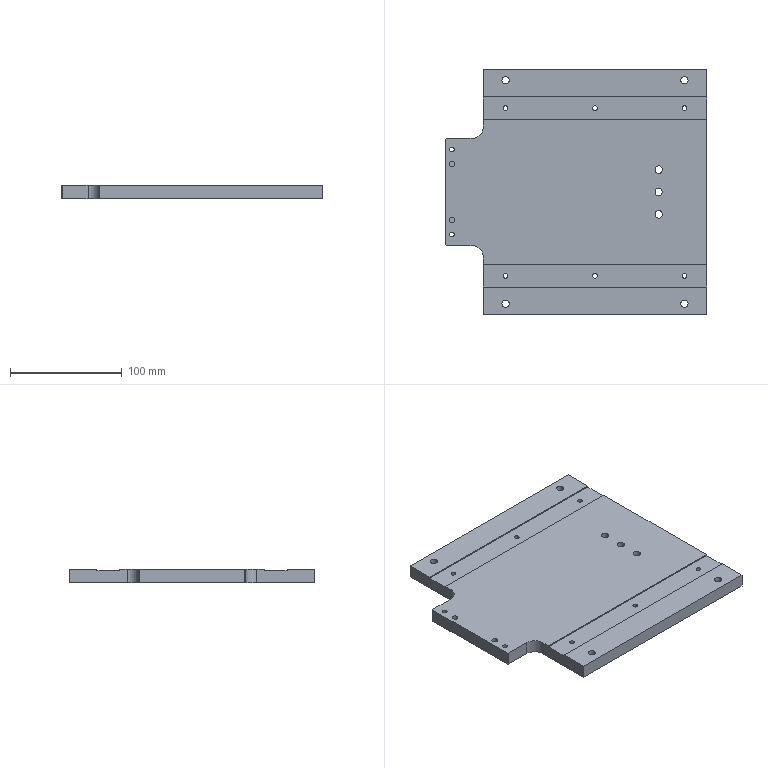Part | STEP file | PN_0078 Mount electronic clip base plate | 1 solid | 67 faces | box 234 x 220 x 12 mm | volume 553966 mm3 | cylinder 42 | plane 25 | commonest cylinder face diameters 4.2 x16 6.5 x8 6.6 x6 11 x6 5 x4 20 x2